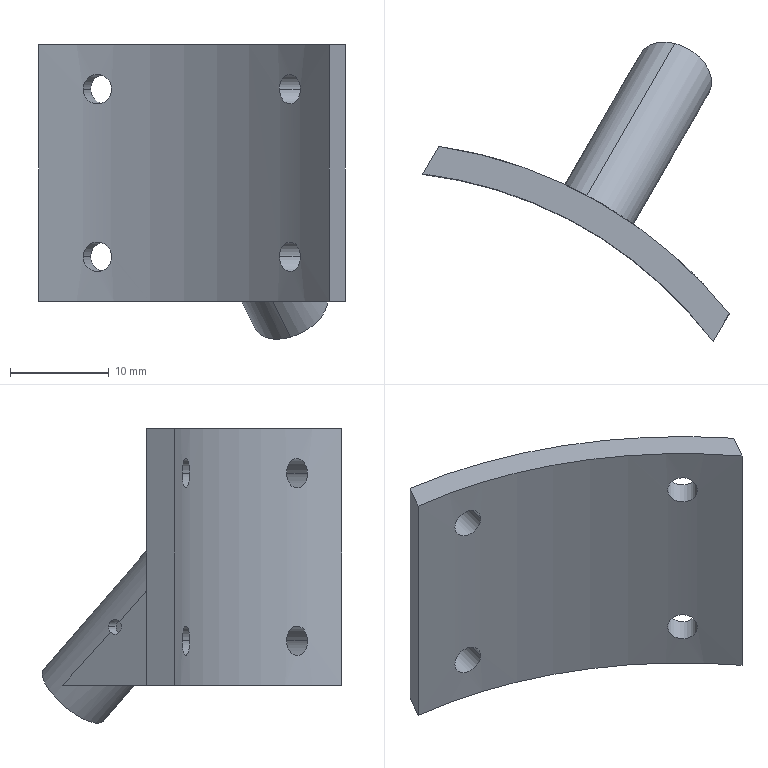Part | SolidWorks | features ICE 5, CirPattern 1, Extrusion 1 | 1 solid | 26 faces | box 31.064 x 30.415 x 29.867 mm | volume 3679 mm3 | cylinder 19 | plane 7 | commonest cylinder face diameters 3 x8 1.5 x4 5 x2 8 x2 93.2 x2 87.2 x1